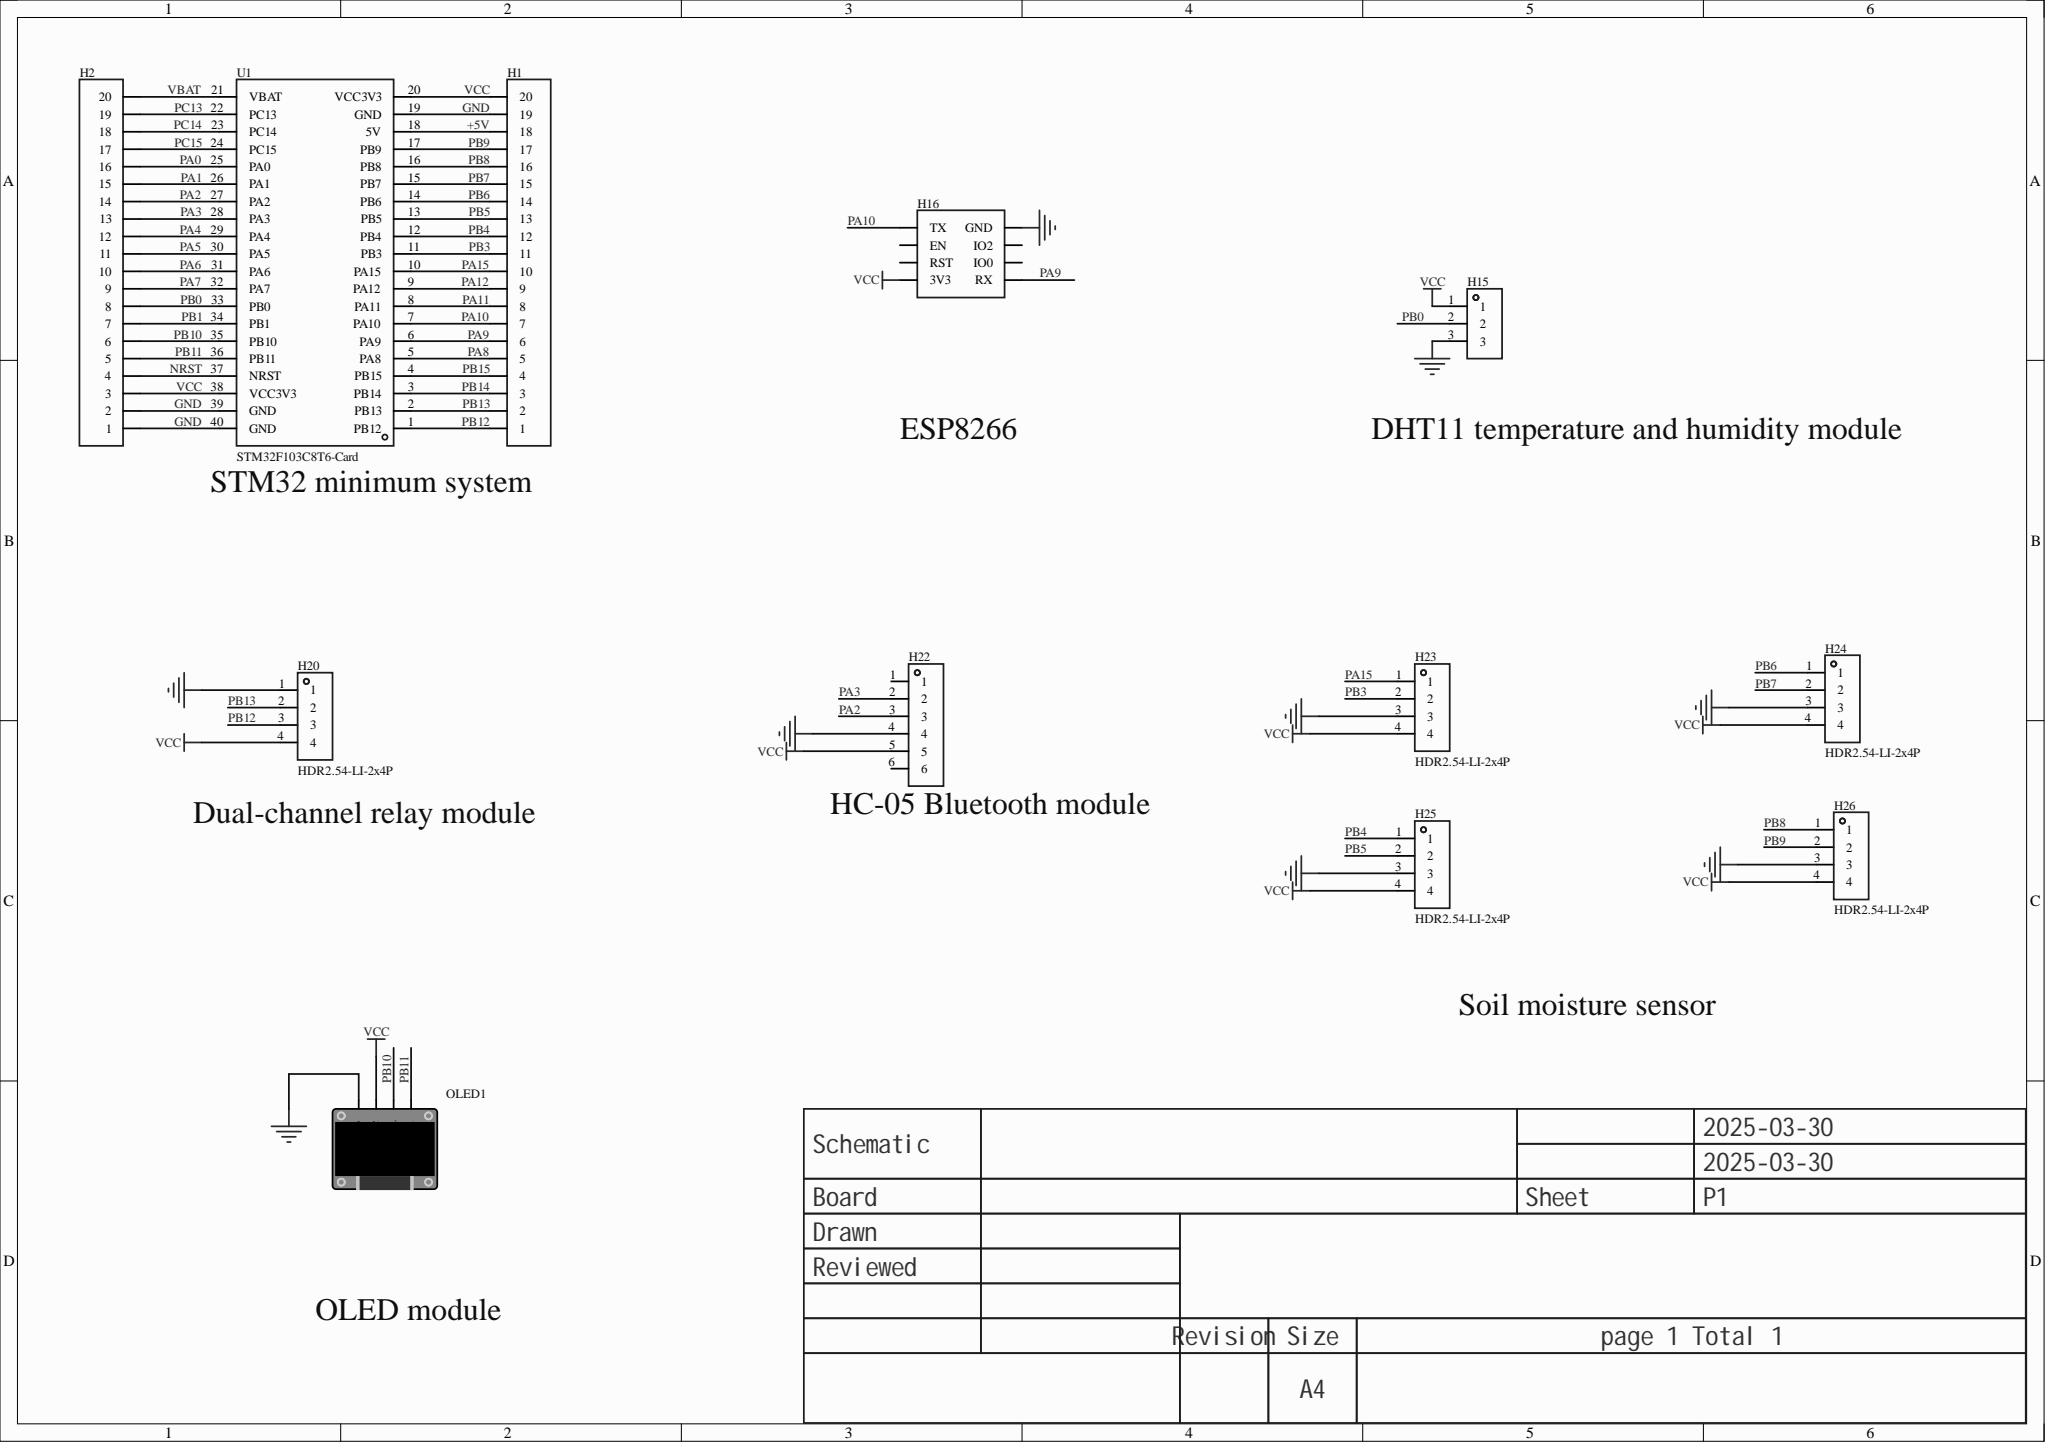Circuit board | Altium Designer | 12 parts | 37 nets
Bill of materials:
Comment,Description,Designator,Footprint,LibRef,Quantity
"","","H1, H2","HDR-TH_20P-P2.54-V-F","HDR-F_2.54_1x20P","2"
"","","H15","HDR-TH_3P-P2.54-V-F","HDR-F_2.54_1x3P","1"
"","","H16","HDR-TH_8P-P2.54-V-F-R2-C4-S2.54-1","HDR-F_2.54_2x4","1"
"HDR2.54-LI-2x4P","","H20, H23, H24, H25, H26","HDR-TH_4P-P2.54-V-M","HDR2.54-LI-2x4P","5"
"","","H22","HDR-TH_6P-P2.54-V-F","HDR-F_2.54_1x6P","1"
"","","OLED1","0.96OLED_4P","0.96OLED模块_4P","1"
"STM32F103C8T6-Card","","U1","CONN-TH_L53.3-W22.9_STM32F103C8T6-CARD","STM32F103C8T6-Card","1"
Netlist (Protel format):
[
H1
HDR-TH_20P-P2.54-V-F




]
[
H2
HDR-TH_20P-P2.54-V-F




]
[
H15
HDR-TH_3P-P2.54-V-F




]
[
H16
HDR-TH_8P-P2.54-V-F-R2-C4-S2.54-1




]
[
H20
HDR-TH_4P-P2.54-V-M
HDR2.54-LI-2x4P



]
[
H22
HDR-TH_6P-P2.54-V-F




]
[
H23
HDR-TH_4P-P2.54-V-M
HDR2.54-LI-2x4P



]
[
H24
HDR-TH_4P-P2.54-V-M
HDR2.54-LI-2x4P



]
[
H25
HDR-TH_4P-P2.54-V-M
HDR2.54-LI-2x4P



]
[
H26
HDR-TH_4P-P2.54-V-M
HDR2.54-LI-2x4P



]
[
OLED1
0.96OLED_4P




]
[
U1
CONN-TH_L53.3-W22.9_STM32F103C8T6-CARD
STM32F103C8T6-Card



]
(
VCC
H1-20
H2-3
H15-1
H16-7
H20-4
H22-5
H23-4
H24-4
H25-4
H26-4
OLED1-2
U1-20
U1-38
)
(
VBAT
H2-20
U1-21
)
(
PC15
H2-17
U1-24
)
(
PC14
H2-18
U1-23
)
(
PC13
H2-19
U1-22
)
(
PB15
H1-4
U1-4
)
(
PB14
H1-3
U1-3
)
(
PB13
H1-2
H20-2
U1-2
)
(
PB12
H1-1
H20-3
U1-1
)
(
PB11
H2-5
OLED1-4
U1-36
)
(
PB10
H2-6
OLED1-3
U1-35
)
(
PB9
H1-17
H26-2
U1-17
)
(
PB8
H1-16
H26-1
U1-16
)
(
PB7
H1-15
H24-2
U1-15
)
(
PB6
H1-14
H24-1
U1-14
)
(
PB5
H1-13
H25-2
U1-13
)
(
PB4
H1-12
H25-1
U1-12
)
(
PB3
H1-11
H23-2
U1-11
)
(
PB1
H2-7
U1-34
)
(
PB0
H2-8
H15-2
U1-33
)
(
PA15
H1-10
H23-1
U1-10
)
(
PA12
H1-9
U1-9
)
(
PA11
H1-8
U1-8
)
(
PA10
H1-7
H16-1
U1-7
)
(
PA9
H1-6
H16-8
U1-6
)
(
PA8
H1-5
U1-5
)
(
PA7
H2-9
U1-32
)
(
PA6
H2-10
U1-31
)
(
PA5
H2-11
U1-30
)
(
PA4
H2-12
U1-29
)
(
PA3
H2-13
H22-2
U1-28
)
(
PA2
H2-14
H22-3
U1-27
)
(
PA1
H2-15
U1-26
)
(
PA0
H2-16
U1-25
)
(
NRST
H2-4
U1-37
)
(
GND
H1-19
H2-1
H2-2
H15-3
H16-2
H20-1
H22-4
H23-3
H24-3
H25-3
H26-3
OLED1-1
U1-19
U1-39
U1-40
)
(
+5V
H1-18
U1-18
)